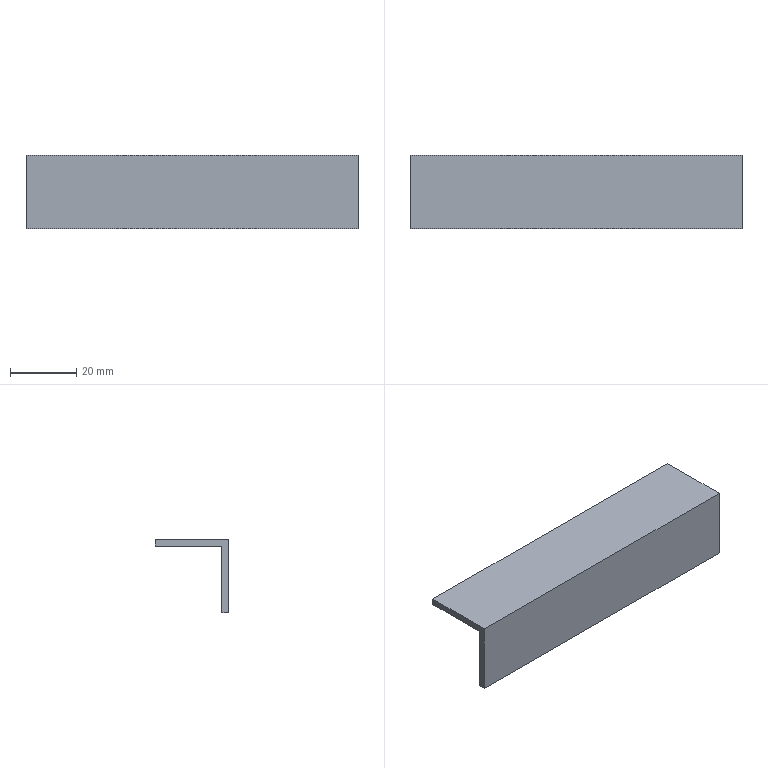Part | NX | 1 solid | 8 faces | box 100 x 22 x 22 mm | volume 8400 mm3 | plane 8
STEP:
#1=CARTESIAN_POINT('',(0.,0.,-20.));
#2=VERTEX_POINT('',#1);
#3=CARTESIAN_POINT('',(0.,0.,0.));
#4=VERTEX_POINT('',#3);
#5=CARTESIAN_POINT('',(0.,0.,0.));
#6=DIRECTION('',(0.,0.,1.));
#7=VECTOR('',#6,1.);
#8=LINE('',#5,#7);
#9=EDGE_CURVE('',#2,#4,#8,.T.);
#10=ORIENTED_EDGE('',*,*,#9,.T.);
#11=CARTESIAN_POINT('',(100.,0.,0.));
#12=VERTEX_POINT('',#11);
#13=CARTESIAN_POINT('',(100.,0.,0.));
#14=DIRECTION('',(-1.,0.,0.));
#15=VECTOR('',#14,1.);
#16=LINE('',#13,#15);
#17=EDGE_CURVE('',#12,#4,#16,.T.);
#18=ORIENTED_EDGE('',*,*,#17,.F.);
#19=CARTESIAN_POINT('',(100.,0.,-20.));
#20=VERTEX_POINT('',#19);
#21=CARTESIAN_POINT('',(100.,0.,0.));
#22=DIRECTION('',(0.,0.,1.));
#23=VECTOR('',#22,1.);
#24=LINE('',#21,#23);
#25=EDGE_CURVE('',#20,#12,#24,.T.);
#26=ORIENTED_EDGE('',*,*,#25,.F.);
#27=CARTESIAN_POINT('',(100.,0.,-20.));
#28=DIRECTION('',(-1.,0.,0.));
#29=VECTOR('',#28,1.);
#30=LINE('',#27,#29);
#31=EDGE_CURVE('',#20,#2,#30,.T.);
#32=ORIENTED_EDGE('',*,*,#31,.T.);
#33=EDGE_LOOP('',(#10,#18,#26,#32));
#34=FACE_OUTER_BOUND('',#33,.T.);
#35=CARTESIAN_POINT('',(100.,0.,0.));
#36=DIRECTION('',(0.,-1.,0.));
#37=DIRECTION('',(0.,0.,-1.));
#38=AXIS2_PLACEMENT_3D('',#35,#36,#37);
#39=PLANE('',#38);
#40=ADVANCED_FACE('',(#34),#39,.F.);
#41=CARTESIAN_POINT('',(0.,20.,0.));
#42=VERTEX_POINT('',#41);
#43=CARTESIAN_POINT('',(0.,0.,0.));
#44=DIRECTION('',(0.,1.,0.));
#45=VECTOR('',#44,1.);
#46=LINE('',#43,#45);
#47=EDGE_CURVE('',#4,#42,#46,.T.);
#48=ORIENTED_EDGE('',*,*,#47,.T.);
#49=CARTESIAN_POINT('',(100.,20.,0.));
#50=VERTEX_POINT('',#49);
#51=CARTESIAN_POINT('',(100.,20.,0.));
#52=DIRECTION('',(-1.,0.,0.));
#53=VECTOR('',#52,1.);
#54=LINE('',#51,#53);
#55=EDGE_CURVE('',#50,#42,#54,.T.);
#56=ORIENTED_EDGE('',*,*,#55,.F.);
#57=CARTESIAN_POINT('',(100.,0.,0.));
#58=DIRECTION('',(0.,1.,0.));
#59=VECTOR('',#58,1.);
#60=LINE('',#57,#59);
#61=EDGE_CURVE('',#12,#50,#60,.T.);
#62=ORIENTED_EDGE('',*,*,#61,.F.);
#63=ORIENTED_EDGE('',*,*,#17,.T.);
#64=EDGE_LOOP('',(#48,#56,#62,#63));
#65=FACE_OUTER_BOUND('',#64,.T.);
#66=CARTESIAN_POINT('',(100.,0.,0.));
#67=DIRECTION('',(0.,0.,1.));
#68=DIRECTION('',(1.,0.,0.));
#69=AXIS2_PLACEMENT_3D('',#66,#67,#68);
#70=PLANE('',#69);
#71=ADVANCED_FACE('',(#65),#70,.F.);
#72=CARTESIAN_POINT('',(0.,20.,2.));
#73=VERTEX_POINT('',#72);
#74=CARTESIAN_POINT('',(0.,20.,2.));
#75=DIRECTION('',(0.,0.,1.));
#76=VECTOR('',#75,1.);
#77=LINE('',#74,#76);
#78=EDGE_CURVE('',#42,#73,#77,.T.);
#79=ORIENTED_EDGE('',*,*,#78,.T.);
#80=CARTESIAN_POINT('',(100.,20.,2.));
#81=VERTEX_POINT('',#80);
#82=CARTESIAN_POINT('',(100.,20.,2.));
#83=DIRECTION('',(-1.,0.,0.));
#84=VECTOR('',#83,1.);
#85=LINE('',#82,#84);
#86=EDGE_CURVE('',#81,#73,#85,.T.);
#87=ORIENTED_EDGE('',*,*,#86,.F.);
#88=CARTESIAN_POINT('',(100.,20.,2.));
#89=DIRECTION('',(0.,0.,1.));
#90=VECTOR('',#89,1.);
#91=LINE('',#88,#90);
#92=EDGE_CURVE('',#50,#81,#91,.T.);
#93=ORIENTED_EDGE('',*,*,#92,.F.);
#94=ORIENTED_EDGE('',*,*,#55,.T.);
#95=EDGE_LOOP('',(#79,#87,#93,#94));
#96=FACE_OUTER_BOUND('',#95,.T.);
#97=CARTESIAN_POINT('',(100.,20.,2.));
#98=DIRECTION('',(0.,-1.,0.));
#99=DIRECTION('',(0.,0.,-1.));
#100=AXIS2_PLACEMENT_3D('',#97,#98,#99);
#101=PLANE('',#100);
#102=ADVANCED_FACE('',(#96),#101,.F.);
#103=CARTESIAN_POINT('',(0.,-2.,2.));
#104=VERTEX_POINT('',#103);
#105=CARTESIAN_POINT('',(0.,-2.,2.));
#106=DIRECTION('',(0.,-1.,0.));
#107=VECTOR('',#106,1.);
#108=LINE('',#105,#107);
#109=EDGE_CURVE('',#73,#104,#108,.T.);
#110=ORIENTED_EDGE('',*,*,#109,.T.);
#111=CARTESIAN_POINT('',(100.,-2.,2.));
#112=VERTEX_POINT('',#111);
#113=CARTESIAN_POINT('',(100.,-2.,2.));
#114=DIRECTION('',(-1.,0.,0.));
#115=VECTOR('',#114,1.);
#116=LINE('',#113,#115);
#117=EDGE_CURVE('',#112,#104,#116,.T.);
#118=ORIENTED_EDGE('',*,*,#117,.F.);
#119=CARTESIAN_POINT('',(100.,-2.,2.));
#120=DIRECTION('',(0.,-1.,0.));
#121=VECTOR('',#120,1.);
#122=LINE('',#119,#121);
#123=EDGE_CURVE('',#81,#112,#122,.T.);
#124=ORIENTED_EDGE('',*,*,#123,.F.);
#125=ORIENTED_EDGE('',*,*,#86,.T.);
#126=EDGE_LOOP('',(#110,#118,#124,#125));
#127=FACE_OUTER_BOUND('',#126,.T.);
#128=CARTESIAN_POINT('',(100.,-2.,2.));
#129=DIRECTION('',(0.,0.,-1.));
#130=DIRECTION('',(-1.,0.,0.));
#131=AXIS2_PLACEMENT_3D('',#128,#129,#130);
#132=PLANE('',#131);
#133=ADVANCED_FACE('',(#127),#132,.F.);
#134=CARTESIAN_POINT('',(0.,-2.,-20.));
#135=VERTEX_POINT('',#134);
#136=CARTESIAN_POINT('',(0.,-2.,2.));
#137=DIRECTION('',(0.,0.,-1.));
#138=VECTOR('',#137,1.);
#139=LINE('',#136,#138);
#140=EDGE_CURVE('',#104,#135,#139,.T.);
#141=ORIENTED_EDGE('',*,*,#140,.T.);
#142=CARTESIAN_POINT('',(100.,-2.,-20.));
#143=VERTEX_POINT('',#142);
#144=CARTESIAN_POINT('',(100.,-2.,-20.));
#145=DIRECTION('',(-1.,0.,0.));
#146=VECTOR('',#145,1.);
#147=LINE('',#144,#146);
#148=EDGE_CURVE('',#143,#135,#147,.T.);
#149=ORIENTED_EDGE('',*,*,#148,.F.);
#150=CARTESIAN_POINT('',(100.,-2.,2.));
#151=DIRECTION('',(0.,0.,-1.));
#152=VECTOR('',#151,1.);
#153=LINE('',#150,#152);
#154=EDGE_CURVE('',#112,#143,#153,.T.);
#155=ORIENTED_EDGE('',*,*,#154,.F.);
#156=ORIENTED_EDGE('',*,*,#117,.T.);
#157=EDGE_LOOP('',(#141,#149,#155,#156));
#158=FACE_OUTER_BOUND('',#157,.T.);
#159=CARTESIAN_POINT('',(100.,-2.,2.));
#160=DIRECTION('',(0.,1.,0.));
#161=DIRECTION('',(0.,0.,1.));
#162=AXIS2_PLACEMENT_3D('',#159,#160,#161);
#163=PLANE('',#162);
#164=ADVANCED_FACE('',(#158),#163,.F.);
#165=CARTESIAN_POINT('',(0.,0.,-20.));
#166=DIRECTION('',(0.,1.,0.));
#167=VECTOR('',#166,1.);
#168=LINE('',#165,#167);
#169=EDGE_CURVE('',#135,#2,#168,.T.);
#170=ORIENTED_EDGE('',*,*,#169,.T.);
#171=ORIENTED_EDGE('',*,*,#31,.F.);
#172=CARTESIAN_POINT('',(100.,0.,-20.));
#173=DIRECTION('',(0.,1.,0.));
#174=VECTOR('',#173,1.);
#175=LINE('',#172,#174);
#176=EDGE_CURVE('',#143,#20,#175,.T.);
#177=ORIENTED_EDGE('',*,*,#176,.F.);
#178=ORIENTED_EDGE('',*,*,#148,.T.);
#179=EDGE_LOOP('',(#170,#171,#177,#178));
#180=FACE_OUTER_BOUND('',#179,.T.);
#181=CARTESIAN_POINT('',(100.,0.,-20.));
#182=DIRECTION('',(0.,0.,1.));
#183=DIRECTION('',(1.,0.,0.));
#184=AXIS2_PLACEMENT_3D('',#181,#182,#183);
#185=PLANE('',#184);
#186=ADVANCED_FACE('',(#180),#185,.F.);
#187=ORIENTED_EDGE('',*,*,#25,.T.);
#188=ORIENTED_EDGE('',*,*,#61,.T.);
#189=ORIENTED_EDGE('',*,*,#92,.T.);
#190=ORIENTED_EDGE('',*,*,#123,.T.);
#191=ORIENTED_EDGE('',*,*,#154,.T.);
#192=ORIENTED_EDGE('',*,*,#176,.T.);
#193=EDGE_LOOP('',(#187,#188,#189,#190,#191,#192));
#194=FACE_OUTER_BOUND('',#193,.T.);
#195=CARTESIAN_POINT('',(100.,0.,-20.));
#196=DIRECTION('',(-1.,0.,0.));
#197=DIRECTION('',(0.,0.,1.));
#198=AXIS2_PLACEMENT_3D('',#195,#196,#197);
#199=PLANE('',#198);
#200=ADVANCED_FACE('',(#194),#199,.F.);
#201=ORIENTED_EDGE('',*,*,#9,.F.);
#202=ORIENTED_EDGE('',*,*,#169,.F.);
#203=ORIENTED_EDGE('',*,*,#140,.F.);
#204=ORIENTED_EDGE('',*,*,#109,.F.);
#205=ORIENTED_EDGE('',*,*,#78,.F.);
#206=ORIENTED_EDGE('',*,*,#47,.F.);
#207=EDGE_LOOP('',(#201,#202,#203,#204,#205,#206));
#208=FACE_OUTER_BOUND('',#207,.T.);
#209=CARTESIAN_POINT('',(0.,0.,-20.));
#210=DIRECTION('',(-1.,0.,0.));
#211=DIRECTION('',(0.,0.,1.));
#212=AXIS2_PLACEMENT_3D('',#209,#210,#211);
#213=PLANE('',#212);
#214=ADVANCED_FACE('',(#208),#213,.T.);
#215=CLOSED_SHELL('',(#40,#71,#102,#133,#164,#186,#200,#214));
#216=MANIFOLD_SOLID_BREP('',#215);
#217=(LENGTH_UNIT()NAMED_UNIT(*)SI_UNIT(.MILLI.,.METRE.));
#218=UNCERTAINTY_MEASURE_WITH_UNIT(LENGTH_MEASURE(0.00002),#217,'','');
#219=(NAMED_UNIT(*)PLANE_ANGLE_UNIT()SI_UNIT($,.RADIAN.));
#220=PLANE_ANGLE_MEASURE_WITH_UNIT(PLANE_ANGLE_MEASURE(0.01745),#219);
#221=DIMENSIONAL_EXPONENTS(0.,0.,0.,0.,0.,0.,0.);
#222=(CONVERSION_BASED_UNIT('DEGREE',#220)NAMED_UNIT(#221)PLANE_ANGLE_UNIT());
#223=(NAMED_UNIT(*)SI_UNIT($,.STERADIAN.)SOLID_ANGLE_UNIT());
#224=(GEOMETRIC_REPRESENTATION_CONTEXT(3)GLOBAL_UNCERTAINTY_ASSIGNED_CONTEXT((#218))GLOBAL_UNIT_ASSIGNED_CONTEXT((#217,#222,#223))REPRESENTATION_CONTEXT('',''));
#225=ADVANCED_BREP_SHAPE_REPRESENTATION('',(#216),#224);